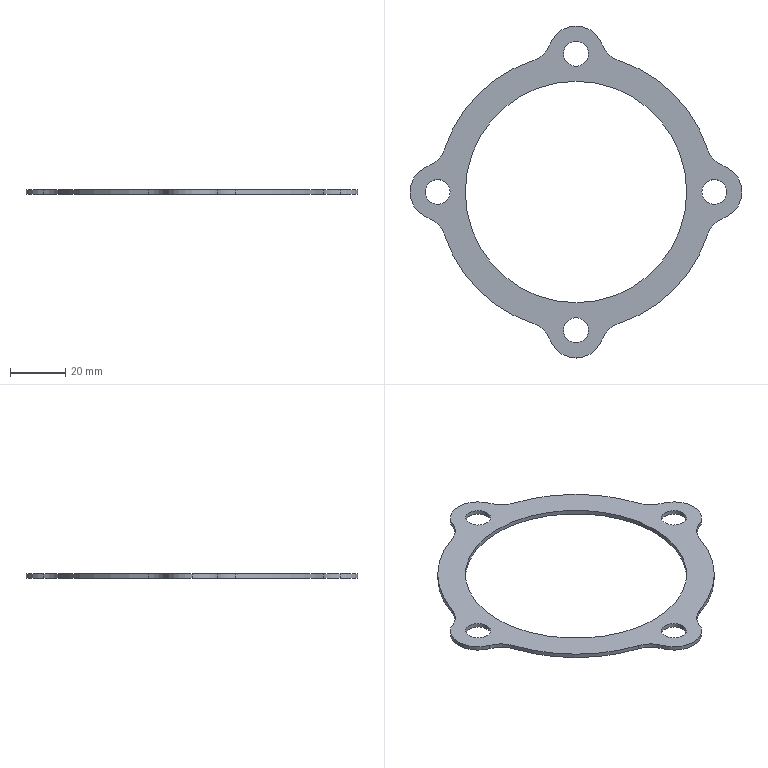Part | SolidWorks | features Extrusion 1 | 1 solid | 29 faces | box 120 x 120 x 1.5 mm | volume 4907 mm3 | cylinder 27 | plane 2 | commonest cylinder face diameters 20 x13 9 x8 100 x4 80 x2
STEP:
#1=CARTESIAN_POINT('',(45.5,0.,1.5));
#2=VERTEX_POINT('',#1);
#3=CARTESIAN_POINT('',(54.5,0.,1.5));
#4=VERTEX_POINT('',#3);
#5=CARTESIAN_POINT('',(50.,0.,1.5));
#6=DIRECTION('',(0.,0.,1.));
#7=DIRECTION('',(1.,0.,0.));
#8=AXIS2_PLACEMENT_3D('',#5,#6,#7);
#9=CIRCLE('',#8,4.5);
#10=EDGE_CURVE('',#2,#4,#9,.T.);
#11=ORIENTED_EDGE('',*,*,#10,.T.);
#12=CARTESIAN_POINT('',(54.5,0.,0.));
#13=VERTEX_POINT('',#12);
#14=CARTESIAN_POINT('',(54.5,0.,1.5));
#15=DIRECTION('',(0.,0.,-1.));
#16=VECTOR('',#15,1000.);
#17=LINE('',#14,#16);
#18=EDGE_CURVE('',#4,#13,#17,.T.);
#19=ORIENTED_EDGE('',*,*,#18,.T.);
#20=CARTESIAN_POINT('',(45.5,0.,0.));
#21=VERTEX_POINT('',#20);
#22=CARTESIAN_POINT('',(50.,0.,0.));
#23=DIRECTION('',(0.,0.,1.));
#24=DIRECTION('',(1.,0.,0.));
#25=AXIS2_PLACEMENT_3D('',#22,#23,#24);
#26=CIRCLE('',#25,4.5);
#27=EDGE_CURVE('',#21,#13,#26,.T.);
#28=ORIENTED_EDGE('',*,*,#27,.F.);
#29=CARTESIAN_POINT('',(45.5,0.,1.5));
#30=DIRECTION('',(0.,0.,-1.));
#31=VECTOR('',#30,1000.);
#32=LINE('',#29,#31);
#33=EDGE_CURVE('',#2,#21,#32,.T.);
#34=ORIENTED_EDGE('',*,*,#33,.F.);
#35=EDGE_LOOP('',(#11,#19,#28,#34));
#36=FACE_OUTER_BOUND('',#35,.T.);
#37=CARTESIAN_POINT('',(50.,0.,1.5));
#38=DIRECTION('',(0.,0.,-1.));
#39=DIRECTION('',(-1.,0.,0.));
#40=AXIS2_PLACEMENT_3D('',#37,#38,#39);
#41=CYLINDRICAL_SURFACE('',#40,4.5);
#42=ADVANCED_FACE('',(#36),#41,.F.);
#43=CARTESIAN_POINT('',(-4.5,-50.,1.5));
#44=VERTEX_POINT('',#43);
#45=CARTESIAN_POINT('',(4.5,-50.,1.5));
#46=VERTEX_POINT('',#45);
#47=CARTESIAN_POINT('',(0.,-50.,1.5));
#48=DIRECTION('',(0.,0.,1.));
#49=DIRECTION('',(1.,0.,0.));
#50=AXIS2_PLACEMENT_3D('',#47,#48,#49);
#51=CIRCLE('',#50,4.5);
#52=EDGE_CURVE('',#44,#46,#51,.T.);
#53=ORIENTED_EDGE('',*,*,#52,.T.);
#54=CARTESIAN_POINT('',(4.5,-50.,0.));
#55=VERTEX_POINT('',#54);
#56=CARTESIAN_POINT('',(4.5,-50.,1.5));
#57=DIRECTION('',(0.,0.,-1.));
#58=VECTOR('',#57,1000.);
#59=LINE('',#56,#58);
#60=EDGE_CURVE('',#46,#55,#59,.T.);
#61=ORIENTED_EDGE('',*,*,#60,.T.);
#62=CARTESIAN_POINT('',(-4.5,-50.,0.));
#63=VERTEX_POINT('',#62);
#64=CARTESIAN_POINT('',(0.,-50.,0.));
#65=DIRECTION('',(0.,0.,1.));
#66=DIRECTION('',(1.,0.,0.));
#67=AXIS2_PLACEMENT_3D('',#64,#65,#66);
#68=CIRCLE('',#67,4.5);
#69=EDGE_CURVE('',#63,#55,#68,.T.);
#70=ORIENTED_EDGE('',*,*,#69,.F.);
#71=CARTESIAN_POINT('',(-4.5,-50.,1.5));
#72=DIRECTION('',(0.,0.,-1.));
#73=VECTOR('',#72,1000.);
#74=LINE('',#71,#73);
#75=EDGE_CURVE('',#44,#63,#74,.T.);
#76=ORIENTED_EDGE('',*,*,#75,.F.);
#77=EDGE_LOOP('',(#53,#61,#70,#76));
#78=FACE_OUTER_BOUND('',#77,.T.);
#79=CARTESIAN_POINT('',(0.,-50.,1.5));
#80=DIRECTION('',(0.,0.,-1.));
#81=DIRECTION('',(-1.,0.,0.));
#82=AXIS2_PLACEMENT_3D('',#79,#80,#81);
#83=CYLINDRICAL_SURFACE('',#82,4.5);
#84=ADVANCED_FACE('',(#78),#83,.F.);
#85=CARTESIAN_POINT('',(-54.5,0.,1.5));
#86=VERTEX_POINT('',#85);
#87=CARTESIAN_POINT('',(-45.5,0.,1.5));
#88=VERTEX_POINT('',#87);
#89=CARTESIAN_POINT('',(-50.,0.,1.5));
#90=DIRECTION('',(0.,0.,1.));
#91=DIRECTION('',(1.,0.,0.));
#92=AXIS2_PLACEMENT_3D('',#89,#90,#91);
#93=CIRCLE('',#92,4.5);
#94=EDGE_CURVE('',#86,#88,#93,.T.);
#95=ORIENTED_EDGE('',*,*,#94,.T.);
#96=CARTESIAN_POINT('',(-45.5,0.,0.));
#97=VERTEX_POINT('',#96);
#98=CARTESIAN_POINT('',(-45.5,0.,1.5));
#99=DIRECTION('',(0.,0.,-1.));
#100=VECTOR('',#99,1000.);
#101=LINE('',#98,#100);
#102=EDGE_CURVE('',#88,#97,#101,.T.);
#103=ORIENTED_EDGE('',*,*,#102,.T.);
#104=CARTESIAN_POINT('',(-54.5,0.,0.));
#105=VERTEX_POINT('',#104);
#106=CARTESIAN_POINT('',(-50.,0.,0.));
#107=DIRECTION('',(0.,0.,1.));
#108=DIRECTION('',(1.,0.,0.));
#109=AXIS2_PLACEMENT_3D('',#106,#107,#108);
#110=CIRCLE('',#109,4.5);
#111=EDGE_CURVE('',#105,#97,#110,.T.);
#112=ORIENTED_EDGE('',*,*,#111,.F.);
#113=CARTESIAN_POINT('',(-54.5,0.,1.5));
#114=DIRECTION('',(0.,0.,-1.));
#115=VECTOR('',#114,1000.);
#116=LINE('',#113,#115);
#117=EDGE_CURVE('',#86,#105,#116,.T.);
#118=ORIENTED_EDGE('',*,*,#117,.F.);
#119=EDGE_LOOP('',(#95,#103,#112,#118));
#120=FACE_OUTER_BOUND('',#119,.T.);
#121=CARTESIAN_POINT('',(-50.,0.,1.5));
#122=DIRECTION('',(0.,0.,-1.));
#123=DIRECTION('',(-1.,0.,0.));
#124=AXIS2_PLACEMENT_3D('',#121,#122,#123);
#125=CYLINDRICAL_SURFACE('',#124,4.5);
#126=ADVANCED_FACE('',(#120),#125,.F.);
#127=CARTESIAN_POINT('',(-4.5,50.,1.5));
#128=VERTEX_POINT('',#127);
#129=CARTESIAN_POINT('',(4.5,50.,1.5));
#130=VERTEX_POINT('',#129);
#131=CARTESIAN_POINT('',(0.,50.,1.5));
#132=DIRECTION('',(0.,0.,1.));
#133=DIRECTION('',(1.,0.,0.));
#134=AXIS2_PLACEMENT_3D('',#131,#132,#133);
#135=CIRCLE('',#134,4.5);
#136=EDGE_CURVE('',#128,#130,#135,.T.);
#137=ORIENTED_EDGE('',*,*,#136,.T.);
#138=CARTESIAN_POINT('',(4.5,50.,0.));
#139=VERTEX_POINT('',#138);
#140=CARTESIAN_POINT('',(4.5,50.,1.5));
#141=DIRECTION('',(0.,0.,-1.));
#142=VECTOR('',#141,1000.);
#143=LINE('',#140,#142);
#144=EDGE_CURVE('',#130,#139,#143,.T.);
#145=ORIENTED_EDGE('',*,*,#144,.T.);
#146=CARTESIAN_POINT('',(-4.5,50.,0.));
#147=VERTEX_POINT('',#146);
#148=CARTESIAN_POINT('',(0.,50.,0.));
#149=DIRECTION('',(0.,0.,1.));
#150=DIRECTION('',(1.,0.,0.));
#151=AXIS2_PLACEMENT_3D('',#148,#149,#150);
#152=CIRCLE('',#151,4.5);
#153=EDGE_CURVE('',#147,#139,#152,.T.);
#154=ORIENTED_EDGE('',*,*,#153,.F.);
#155=CARTESIAN_POINT('',(-4.5,50.,1.5));
#156=DIRECTION('',(0.,0.,-1.));
#157=VECTOR('',#156,1000.);
#158=LINE('',#155,#157);
#159=EDGE_CURVE('',#128,#147,#158,.T.);
#160=ORIENTED_EDGE('',*,*,#159,.F.);
#161=EDGE_LOOP('',(#137,#145,#154,#160));
#162=FACE_OUTER_BOUND('',#161,.T.);
#163=CARTESIAN_POINT('',(0.,50.,1.5));
#164=DIRECTION('',(0.,0.,-1.));
#165=DIRECTION('',(-1.,0.,0.));
#166=AXIS2_PLACEMENT_3D('',#163,#164,#165);
#167=CYLINDRICAL_SURFACE('',#166,4.5);
#168=ADVANCED_FACE('',(#162),#167,.F.);
#169=CARTESIAN_POINT('',(-40.,0.,1.5));
#170=VERTEX_POINT('',#169);
#171=CARTESIAN_POINT('',(40.,0.,1.5));
#172=VERTEX_POINT('',#171);
#173=CARTESIAN_POINT('',(0.,0.,1.5));
#174=DIRECTION('',(0.,0.,1.));
#175=DIRECTION('',(1.,0.,0.));
#176=AXIS2_PLACEMENT_3D('',#173,#174,#175);
#177=CIRCLE('',#176,40.);
#178=EDGE_CURVE('',#170,#172,#177,.T.);
#179=ORIENTED_EDGE('',*,*,#178,.T.);
#180=CARTESIAN_POINT('',(40.,0.,0.));
#181=VERTEX_POINT('',#180);
#182=CARTESIAN_POINT('',(40.,0.,1.5));
#183=DIRECTION('',(0.,0.,-1.));
#184=VECTOR('',#183,1000.);
#185=LINE('',#182,#184);
#186=EDGE_CURVE('',#172,#181,#185,.T.);
#187=ORIENTED_EDGE('',*,*,#186,.T.);
#188=CARTESIAN_POINT('',(-40.,0.,0.));
#189=VERTEX_POINT('',#188);
#190=CARTESIAN_POINT('',(0.,0.,0.));
#191=DIRECTION('',(0.,0.,1.));
#192=DIRECTION('',(1.,0.,0.));
#193=AXIS2_PLACEMENT_3D('',#190,#191,#192);
#194=CIRCLE('',#193,40.);
#195=EDGE_CURVE('',#189,#181,#194,.T.);
#196=ORIENTED_EDGE('',*,*,#195,.F.);
#197=CARTESIAN_POINT('',(-40.,0.,1.5));
#198=DIRECTION('',(0.,0.,-1.));
#199=VECTOR('',#198,1000.);
#200=LINE('',#197,#199);
#201=EDGE_CURVE('',#170,#189,#200,.T.);
#202=ORIENTED_EDGE('',*,*,#201,.F.);
#203=EDGE_LOOP('',(#179,#187,#196,#202));
#204=FACE_OUTER_BOUND('',#203,.T.);
#205=CARTESIAN_POINT('',(0.,0.,1.5));
#206=DIRECTION('',(0.,0.,-1.));
#207=DIRECTION('',(-1.,0.,0.));
#208=AXIS2_PLACEMENT_3D('',#205,#206,#207);
#209=CYLINDRICAL_SURFACE('',#208,40.);
#210=ADVANCED_FACE('',(#204),#209,.F.);
#211=CARTESIAN_POINT('',(-60.,0.,1.5));
#212=VERTEX_POINT('',#211);
#213=CARTESIAN_POINT('',(-53.5,-9.367,1.5));
#214=VERTEX_POINT('',#213);
#215=CARTESIAN_POINT('',(-50.,0.,1.5));
#216=DIRECTION('',(0.,0.,1.));
#217=DIRECTION('',(1.,0.,0.));
#218=AXIS2_PLACEMENT_3D('',#215,#216,#217);
#219=CIRCLE('',#218,10.);
#220=EDGE_CURVE('',#212,#214,#219,.T.);
#221=ORIENTED_EDGE('',*,*,#220,.F.);
#222=CARTESIAN_POINT('',(-60.,0.,0.));
#223=VERTEX_POINT('',#222);
#224=CARTESIAN_POINT('',(-60.,0.,1.5));
#225=DIRECTION('',(0.,0.,-1.));
#226=VECTOR('',#225,1000.);
#227=LINE('',#224,#226);
#228=EDGE_CURVE('',#212,#223,#227,.T.);
#229=ORIENTED_EDGE('',*,*,#228,.T.);
#230=CARTESIAN_POINT('',(-53.5,-9.367,0.));
#231=VERTEX_POINT('',#230);
#232=CARTESIAN_POINT('',(-50.,0.,0.));
#233=DIRECTION('',(0.,0.,1.));
#234=DIRECTION('',(1.,0.,0.));
#235=AXIS2_PLACEMENT_3D('',#232,#233,#234);
#236=CIRCLE('',#235,10.);
#237=EDGE_CURVE('',#223,#231,#236,.T.);
#238=ORIENTED_EDGE('',*,*,#237,.T.);
#239=CARTESIAN_POINT('',(-53.5,-9.367,1.5));
#240=DIRECTION('',(0.,0.,-1.));
#241=VECTOR('',#240,1000.);
#242=LINE('',#239,#241);
#243=EDGE_CURVE('',#214,#231,#242,.T.);
#244=ORIENTED_EDGE('',*,*,#243,.F.);
#245=EDGE_LOOP('',(#221,#229,#238,#244));
#246=FACE_OUTER_BOUND('',#245,.T.);
#247=CARTESIAN_POINT('',(-50.,0.,1.5));
#248=DIRECTION('',(0.,0.,-1.));
#249=DIRECTION('',(-1.,0.,0.));
#250=AXIS2_PLACEMENT_3D('',#247,#248,#249);
#251=CYLINDRICAL_SURFACE('',#250,10.);
#252=ADVANCED_FACE('',(#246),#251,.T.);
#253=ORIENTED_EDGE('',*,*,#52,.F.);
#254=CARTESIAN_POINT('',(0.,-50.,1.5));
#255=DIRECTION('',(0.,0.,1.));
#256=DIRECTION('',(1.,0.,0.));
#257=AXIS2_PLACEMENT_3D('',#254,#255,#256);
#258=CIRCLE('',#257,4.5);
#259=EDGE_CURVE('',#46,#44,#258,.T.);
#260=ORIENTED_EDGE('',*,*,#259,.F.);
#261=EDGE_LOOP('',(#253,#260));
#262=FACE_BOUND('',#261,.T.);
#263=ORIENTED_EDGE('',*,*,#136,.F.);
#264=CARTESIAN_POINT('',(0.,50.,1.5));
#265=DIRECTION('',(0.,0.,1.));
#266=DIRECTION('',(1.,0.,0.));
#267=AXIS2_PLACEMENT_3D('',#264,#265,#266);
#268=CIRCLE('',#267,4.5);
#269=EDGE_CURVE('',#130,#128,#268,.T.);
#270=ORIENTED_EDGE('',*,*,#269,.F.);
#271=EDGE_LOOP('',(#263,#270));
#272=FACE_BOUND('',#271,.T.);
#273=CARTESIAN_POINT('',(-9.367,53.5,1.5));
#274=VERTEX_POINT('',#273);
#275=CARTESIAN_POINT('',(-15.612,47.5,1.5));
#276=VERTEX_POINT('',#275);
#277=CARTESIAN_POINT('',(-18.735,57.,1.5));
#278=DIRECTION('',(0.,0.,-1.));
#279=DIRECTION('',(1.,0.,0.));
#280=AXIS2_PLACEMENT_3D('',#277,#278,#279);
#281=CIRCLE('',#280,10.);
#282=EDGE_CURVE('',#274,#276,#281,.T.);
#283=ORIENTED_EDGE('',*,*,#282,.T.);
#284=CARTESIAN_POINT('',(-47.5,15.612,1.5));
#285=VERTEX_POINT('',#284);
#286=CARTESIAN_POINT('',(0.,0.,1.5));
#287=DIRECTION('',(0.,0.,1.));
#288=DIRECTION('',(1.,0.,0.));
#289=AXIS2_PLACEMENT_3D('',#286,#287,#288);
#290=CIRCLE('',#289,50.);
#291=EDGE_CURVE('',#276,#285,#290,.T.);
#292=ORIENTED_EDGE('',*,*,#291,.T.);
#293=CARTESIAN_POINT('',(-53.5,9.367,1.5));
#294=VERTEX_POINT('',#293);
#295=CARTESIAN_POINT('',(-57.,18.735,1.5));
#296=DIRECTION('',(0.,0.,-1.));
#297=DIRECTION('',(-1.,0.,0.));
#298=AXIS2_PLACEMENT_3D('',#295,#296,#297);
#299=CIRCLE('',#298,10.);
#300=EDGE_CURVE('',#285,#294,#299,.T.);
#301=ORIENTED_EDGE('',*,*,#300,.T.);
#302=CARTESIAN_POINT('',(-50.,0.,1.5));
#303=DIRECTION('',(0.,0.,1.));
#304=DIRECTION('',(1.,0.,0.));
#305=AXIS2_PLACEMENT_3D('',#302,#303,#304);
#306=CIRCLE('',#305,10.);
#307=EDGE_CURVE('',#294,#212,#306,.T.);
#308=ORIENTED_EDGE('',*,*,#307,.T.);
#309=ORIENTED_EDGE('',*,*,#220,.T.);
#310=CARTESIAN_POINT('',(-47.5,-15.612,1.5));
#311=VERTEX_POINT('',#310);
#312=CARTESIAN_POINT('',(-57.,-18.735,1.5));
#313=DIRECTION('',(0.,0.,-1.));
#314=DIRECTION('',(-1.,0.,0.));
#315=AXIS2_PLACEMENT_3D('',#312,#313,#314);
#316=CIRCLE('',#315,10.);
#317=EDGE_CURVE('',#214,#311,#316,.T.);
#318=ORIENTED_EDGE('',*,*,#317,.T.);
#319=CARTESIAN_POINT('',(-15.612,-47.5,1.5));
#320=VERTEX_POINT('',#319);
#321=CARTESIAN_POINT('',(0.,0.,1.5));
#322=DIRECTION('',(0.,0.,1.));
#323=DIRECTION('',(1.,0.,0.));
#324=AXIS2_PLACEMENT_3D('',#321,#322,#323);
#325=CIRCLE('',#324,50.);
#326=EDGE_CURVE('',#311,#320,#325,.T.);
#327=ORIENTED_EDGE('',*,*,#326,.T.);
#328=CARTESIAN_POINT('',(-9.367,-53.5,1.5));
#329=VERTEX_POINT('',#328);
#330=CARTESIAN_POINT('',(-18.735,-57.,1.5));
#331=DIRECTION('',(0.,0.,-1.));
#332=DIRECTION('',(-1.,0.,0.));
#333=AXIS2_PLACEMENT_3D('',#330,#331,#332);
#334=CIRCLE('',#333,10.);
#335=EDGE_CURVE('',#320,#329,#334,.T.);
#336=ORIENTED_EDGE('',*,*,#335,.T.);
#337=CARTESIAN_POINT('',(9.367,-53.5,1.5));
#338=VERTEX_POINT('',#337);
#339=CARTESIAN_POINT('',(0.,-50.,1.5));
#340=DIRECTION('',(0.,0.,1.));
#341=DIRECTION('',(1.,0.,0.));
#342=AXIS2_PLACEMENT_3D('',#339,#340,#341);
#343=CIRCLE('',#342,10.);
#344=EDGE_CURVE('',#329,#338,#343,.T.);
#345=ORIENTED_EDGE('',*,*,#344,.T.);
#346=CARTESIAN_POINT('',(15.612,-47.5,1.5));
#347=VERTEX_POINT('',#346);
#348=CARTESIAN_POINT('',(18.735,-57.,1.5));
#349=DIRECTION('',(0.,0.,-1.));
#350=DIRECTION('',(-1.,0.,0.));
#351=AXIS2_PLACEMENT_3D('',#348,#349,#350);
#352=CIRCLE('',#351,10.);
#353=EDGE_CURVE('',#338,#347,#352,.T.);
#354=ORIENTED_EDGE('',*,*,#353,.T.);
#355=CARTESIAN_POINT('',(47.5,-15.612,1.5));
#356=VERTEX_POINT('',#355);
#357=CARTESIAN_POINT('',(0.,0.,1.5));
#358=DIRECTION('',(0.,0.,1.));
#359=DIRECTION('',(1.,0.,0.));
#360=AXIS2_PLACEMENT_3D('',#357,#358,#359);
#361=CIRCLE('',#360,50.);
#362=EDGE_CURVE('',#347,#356,#361,.T.);
#363=ORIENTED_EDGE('',*,*,#362,.T.);
#364=CARTESIAN_POINT('',(53.5,-9.367,1.5));
#365=VERTEX_POINT('',#364);
#366=CARTESIAN_POINT('',(57.,-18.735,1.5));
#367=DIRECTION('',(0.,0.,-1.));
#368=DIRECTION('',(-1.,0.,0.));
#369=AXIS2_PLACEMENT_3D('',#366,#367,#368);
#370=CIRCLE('',#369,10.);
#371=EDGE_CURVE('',#356,#365,#370,.T.);
#372=ORIENTED_EDGE('',*,*,#371,.T.);
#373=CARTESIAN_POINT('',(53.5,9.367,1.5));
#374=VERTEX_POINT('',#373);
#375=CARTESIAN_POINT('',(50.,0.,1.5));
#376=DIRECTION('',(0.,0.,1.));
#377=DIRECTION('',(1.,0.,0.));
#378=AXIS2_PLACEMENT_3D('',#375,#376,#377);
#379=CIRCLE('',#378,10.);
#380=EDGE_CURVE('',#365,#374,#379,.T.);
#381=ORIENTED_EDGE('',*,*,#380,.T.);
#382=CARTESIAN_POINT('',(47.5,15.612,1.5));
#383=VERTEX_POINT('',#382);
#384=CARTESIAN_POINT('',(57.,18.735,1.5));
#385=DIRECTION('',(0.,0.,-1.));
#386=DIRECTION('',(-1.,0.,0.));
#387=AXIS2_PLACEMENT_3D('',#384,#385,#386);
#388=CIRCLE('',#387,10.);
#389=EDGE_CURVE('',#374,#383,#388,.T.);
#390=ORIENTED_EDGE('',*,*,#389,.T.);
#391=CARTESIAN_POINT('',(15.612,47.5,1.5));
#392=VERTEX_POINT('',#391);
#393=CARTESIAN_POINT('',(0.,0.,1.5));
#394=DIRECTION('',(0.,0.,1.));
#395=DIRECTION('',(1.,0.,0.));
#396=AXIS2_PLACEMENT_3D('',#393,#394,#395);
#397=CIRCLE('',#396,50.);
#398=EDGE_CURVE('',#383,#392,#397,.T.);
#399=ORIENTED_EDGE('',*,*,#398,.T.);
#400=CARTESIAN_POINT('',(9.367,53.5,1.5));
#401=VERTEX_POINT('',#400);
#402=CARTESIAN_POINT('',(18.735,57.,1.5));
#403=DIRECTION('',(0.,0.,-1.));
#404=DIRECTION('',(-1.,0.,0.));
#405=AXIS2_PLACEMENT_3D('',#402,#403,#404);
#406=CIRCLE('',#405,10.);
#407=EDGE_CURVE('',#392,#401,#406,.T.);
#408=ORIENTED_EDGE('',*,*,#407,.T.);
#409=CARTESIAN_POINT('',(0.,50.,1.5));
#410=DIRECTION('',(0.,0.,1.));
#411=DIRECTION('',(1.,0.,0.));
#412=AXIS2_PLACEMENT_3D('',#409,#410,#411);
#413=CIRCLE('',#412,10.);
#414=EDGE_CURVE('',#401,#274,#413,.T.);
#415=ORIENTED_EDGE('',*,*,#414,.T.);
#416=EDGE_LOOP('',(#283,#292,#301,#308,#309,#318,#327,#336,#345,#354,#363,#372,#381,#390,#399,#408,#415));
#417=FACE_OUTER_BOUND('',#416,.T.);
#418=ORIENTED_EDGE('',*,*,#178,.F.);
#419=CARTESIAN_POINT('',(0.,0.,1.5));
#420=DIRECTION('',(0.,0.,1.));
#421=DIRECTION('',(1.,0.,0.));
#422=AXIS2_PLACEMENT_3D('',#419,#420,#421);
#423=CIRCLE('',#422,40.);
#424=EDGE_CURVE('',#172,#170,#423,.T.);
#425=ORIENTED_EDGE('',*,*,#424,.F.);
#426=EDGE_LOOP('',(#418,#425));
#427=FACE_BOUND('',#426,.T.);
#428=ORIENTED_EDGE('',*,*,#94,.F.);
#429=CARTESIAN_POINT('',(-50.,0.,1.5));
#430=DIRECTION('',(0.,0.,1.));
#431=DIRECTION('',(1.,0.,0.));
#432=AXIS2_PLACEMENT_3D('',#429,#430,#431);
#433=CIRCLE('',#432,4.5);
#434=EDGE_CURVE('',#88,#86,#433,.T.);
#435=ORIENTED_EDGE('',*,*,#434,.F.);
#436=EDGE_LOOP('',(#428,#435));
#437=FACE_BOUND('',#436,.T.);
#438=ORIENTED_EDGE('',*,*,#10,.F.);
#439=CARTESIAN_POINT('',(50.,0.,1.5));
#440=DIRECTION('',(0.,0.,1.));
#441=DIRECTION('',(1.,0.,0.));
#442=AXIS2_PLACEMENT_3D('',#439,#440,#441);
#443=CIRCLE('',#442,4.5);
#444=EDGE_CURVE('',#4,#2,#443,.T.);
#445=ORIENTED_EDGE('',*,*,#444,.F.);
#446=EDGE_LOOP('',(#438,#445));
#447=FACE_BOUND('',#446,.T.);
#448=CARTESIAN_POINT('',(-9.367,53.5,1.5));
#449=DIRECTION('',(0.,0.,1.));
#450=DIRECTION('',(1.,0.,0.));
#451=AXIS2_PLACEMENT_3D('',#448,#449,#450);
#452=PLANE('',#451);
#453=ADVANCED_FACE('',(#262,#272,#417,#427,#437,#447),#452,.T.);
#454=CARTESIAN_POINT('',(-9.367,53.5,0.));
#455=VERTEX_POINT('',#454);
#456=CARTESIAN_POINT('',(-15.612,47.5,0.));
#457=VERTEX_POINT('',#456);
#458=CARTESIAN_POINT('',(-18.735,57.,0.));
#459=DIRECTION('',(0.,0.,-1.));
#460=DIRECTION('',(1.,0.,0.));
#461=AXIS2_PLACEMENT_3D('',#458,#459,#460);
#462=CIRCLE('',#461,10.);
#463=EDGE_CURVE('',#455,#457,#462,.T.);
#464=ORIENTED_EDGE('',*,*,#463,.F.);
#465=CARTESIAN_POINT('',(9.367,53.5,0.));
#466=VERTEX_POINT('',#465);
#467=CARTESIAN_POINT('',(0.,50.,0.));
#468=DIRECTION('',(0.,0.,1.));
#469=DIRECTION('',(1.,0.,0.));
#470=AXIS2_PLACEMENT_3D('',#467,#468,#469);
#471=CIRCLE('',#470,10.);
#472=EDGE_CURVE('',#466,#455,#471,.T.);
#473=ORIENTED_EDGE('',*,*,#472,.F.);
#474=CARTESIAN_POINT('',(15.612,47.5,0.));
#475=VERTEX_POINT('',#474);
#476=CARTESIAN_POINT('',(18.735,57.,0.));
#477=DIRECTION('',(0.,0.,-1.));
#478=DIRECTION('',(-1.,0.,0.));
#479=AXIS2_PLACEMENT_3D('',#476,#477,#478);
#480=CIRCLE('',#479,10.);
#481=EDGE_CURVE('',#475,#466,#480,.T.);
#482=ORIENTED_EDGE('',*,*,#481,.F.);
#483=CARTESIAN_POINT('',(47.5,15.612,0.));
#484=VERTEX_POINT('',#483);
#485=CARTESIAN_POINT('',(0.,0.,0.));
#486=DIRECTION('',(0.,0.,1.));
#487=DIRECTION('',(1.,0.,0.));
#488=AXIS2_PLACEMENT_3D('',#485,#486,#487);
#489=CIRCLE('',#488,50.);
#490=EDGE_CURVE('',#484,#475,#489,.T.);
#491=ORIENTED_EDGE('',*,*,#490,.F.);
#492=CARTESIAN_POINT('',(53.5,9.367,0.));
#493=VERTEX_POINT('',#492);
#494=CARTESIAN_POINT('',(57.,18.735,0.));
#495=DIRECTION('',(0.,0.,-1.));
#496=DIRECTION('',(-1.,0.,0.));
#497=AXIS2_PLACEMENT_3D('',#494,#495,#496);
#498=CIRCLE('',#497,10.);
#499=EDGE_CURVE('',#493,#484,#498,.T.);
#500=ORIENTED_EDGE('',*,*,#499,.F.);
#501=CARTESIAN_POINT('',(53.5,-9.367,0.));
#502=VERTEX_POINT('',#501);
#503=CARTESIAN_POINT('',(50.,0.,0.));
#504=DIRECTION('',(0.,0.,1.));
#505=DIRECTION('',(1.,0.,0.));
#506=AXIS2_PLACEMENT_3D('',#503,#504,#505);
#507=CIRCLE('',#506,10.);
#508=EDGE_CURVE('',#502,#493,#507,.T.);
#509=ORIENTED_EDGE('',*,*,#508,.F.);
#510=CARTESIAN_POINT('',(47.5,-15.612,0.));
#511=VERTEX_POINT('',#510);
#512=CARTESIAN_POINT('',(57.,-18.735,0.));
#513=DIRECTION('',(0.,0.,-1.));
#514=DIRECTION('',(-1.,0.,0.));
#515=AXIS2_PLACEMENT_3D('',#512,#513,#514);
#516=CIRCLE('',#515,10.);
#517=EDGE_CURVE('',#511,#502,#516,.T.);
#518=ORIENTED_EDGE('',*,*,#517,.F.);
#519=CARTESIAN_POINT('',(15.612,-47.5,0.));
#520=VERTEX_POINT('',#519);
#521=CARTESIAN_POINT('',(0.,0.,0.));
#522=DIRECTION('',(0.,0.,1.));
#523=DIRECTION('',(1.,0.,0.));
#524=AXIS2_PLACEMENT_3D('',#521,#522,#523);
#525=CIRCLE('',#524,50.);
#526=EDGE_CURVE('',#520,#511,#525,.T.);
#527=ORIENTED_EDGE('',*,*,#526,.F.);
#528=CARTESIAN_POINT('',(9.367,-53.5,0.));
#529=VERTEX_POINT('',#528);
#530=CARTESIAN_POINT('',(18.735,-57.,0.));
#531=DIRECTION('',(0.,0.,-1.));
#532=DIRECTION('',(-1.,0.,0.));
#533=AXIS2_PLACEMENT_3D('',#530,#531,#532);
#534=CIRCLE('',#533,10.);
#535=EDGE_CURVE('',#529,#520,#534,.T.);
#536=ORIENTED_EDGE('',*,*,#535,.F.);
#537=CARTESIAN_POINT('',(-9.367,-53.5,0.));
#538=VERTEX_POINT('',#537);
#539=CARTESIAN_POINT('',(0.,-50.,0.));
#540=DIRECTION('',(0.,0.,1.));
#541=DIRECTION('',(1.,0.,0.));
#542=AXIS2_PLACEMENT_3D('',#539,#540,#541);
#543=CIRCLE('',#542,10.);
#544=EDGE_CURVE('',#538,#529,#543,.T.);
#545=ORIENTED_EDGE('',*,*,#544,.F.);
#546=CARTESIAN_POINT('',(-15.612,-47.5,0.));
#547=VERTEX_POINT('',#546);
#548=CARTESIAN_POINT('',(-18.735,-57.,0.));
#549=DIRECTION('',(0.,0.,-1.));
#550=DIRECTION('',(-1.,0.,0.));
#551=AXIS2_PLACEMENT_3D('',#548,#549,#550);
#552=CIRCLE('',#551,10.);
#553=EDGE_CURVE('',#547,#538,#552,.T.);
#554=ORIENTED_EDGE('',*,*,#553,.F.);
#555=CARTESIAN_POINT('',(-47.5,-15.612,0.));
#556=VERTEX_POINT('',#555);
#557=CARTESIAN_POINT('',(0.,0.,0.));
#558=DIRECTION('',(0.,0.,1.));
#559=DIRECTION('',(1.,0.,0.));
#560=AXIS2_PLACEMENT_3D('',#557,#558,#559);
#561=CIRCLE('',#560,50.);
#562=EDGE_CURVE('',#556,#547,#561,.T.);
#563=ORIENTED_EDGE('',*,*,#562,.F.);
#564=CARTESIAN_POINT('',(-57.,-18.735,0.));
#565=DIRECTION('',(0.,0.,-1.));
#566=DIRECTION('',(-1.,0.,0.));
#567=AXIS2_PLACEMENT_3D('',#564,#565,#566);
#568=CIRCLE('',#567,10.);
#569=EDGE_CURVE('',#231,#556,#568,.T.);
#570=ORIENTED_EDGE('',*,*,#569,.F.);
#571=ORIENTED_EDGE('',*,*,#237,.F.);
#572=CARTESIAN_POINT('',(-53.5,9.367,0.));
#573=VERTEX_POINT('',#572);
#574=CARTESIAN_POINT('',(-50.,0.,0.));
#575=DIRECTION('',(0.,0.,1.));
#576=DIRECTION('',(1.,0.,0.));
#577=AXIS2_PLACEMENT_3D('',#574,#575,#576);
#578=CIRCLE('',#577,10.);
#579=EDGE_CURVE('',#573,#223,#578,.T.);
#580=ORIENTED_EDGE('',*,*,#579,.F.);
#581=CARTESIAN_POINT('',(-47.5,15.612,0.));
#582=VERTEX_POINT('',#581);
#583=CARTESIAN_POINT('',(-57.,18.735,0.));
#584=DIRECTION('',(0.,0.,-1.));
#585=DIRECTION('',(-1.,0.,0.));
#586=AXIS2_PLACEMENT_3D('',#583,#584,#585);
#587=CIRCLE('',#586,10.);
#588=EDGE_CURVE('',#582,#573,#587,.T.);
#589=ORIENTED_EDGE('',*,*,#588,.F.);
#590=CARTESIAN_POINT('',(0.,0.,0.));
#591=DIRECTION('',(0.,0.,1.));
#592=DIRECTION('',(1.,0.,0.));
#593=AXIS2_PLACEMENT_3D('',#590,#591,#592);
#594=CIRCLE('',#593,50.);
#595=EDGE_CURVE('',#457,#582,#594,.T.);
#596=ORIENTED_EDGE('',*,*,#595,.F.);
#597=EDGE_LOOP('',(#464,#473,#482,#491,#500,#509,#518,#527,#536,#545,#554,#563,#570,#571,#580,#589,#596));
#598=FACE_OUTER_BOUND('',#597,.T.);
#599=ORIENTED_EDGE('',*,*,#195,.T.);
#600=CARTESIAN_POINT('',(0.,0.,0.));
#601=DIRECTION('',(0.,0.,1.));
#602=DIRECTION('',(1.,0.,0.));
#603=AXIS2_PLACEMENT_3D('',#600,#601,#602);
#604=CIRCLE('',#603,40.);
#605=EDGE_CURVE('',#181,#189,#604,.T.);
#606=ORIENTED_EDGE('',*,*,#605,.T.);
#607=EDGE_LOOP('',(#599,#606));
#608=FACE_BOUND('',#607,.T.);
#609=ORIENTED_EDGE('',*,*,#153,.T.);
#610=CARTESIAN_POINT('',(0.,50.,0.));
#611=DIRECTION('',(0.,0.,1.));
#612=DIRECTION('',(1.,0.,0.));
#613=AXIS2_PLACEMENT_3D('',#610,#611,#612);
#614=CIRCLE('',#613,4.5);
#615=EDGE_CURVE('',#139,#147,#614,.T.);
#616=ORIENTED_EDGE('',*,*,#615,.T.);
#617=EDGE_LOOP('',(#609,#616));
#618=FACE_BOUND('',#617,.T.);
#619=ORIENTED_EDGE('',*,*,#111,.T.);
#620=CARTESIAN_POINT('',(-50.,0.,0.));
#621=DIRECTION('',(0.,0.,1.));
#622=DIRECTION('',(1.,0.,0.));
#623=AXIS2_PLACEMENT_3D('',#620,#621,#622);
#624=CIRCLE('',#623,4.5);
#625=EDGE_CURVE('',#97,#105,#624,.T.);
#626=ORIENTED_EDGE('',*,*,#625,.T.);
#627=EDGE_LOOP('',(#619,#626));
#628=FACE_BOUND('',#627,.T.);
#629=ORIENTED_EDGE('',*,*,#69,.T.);
#630=CARTESIAN_POINT('',(0.,-50.,0.));
#631=DIRECTION('',(0.,0.,1.));
#632=DIRECTION('',(1.,0.,0.));
#633=AXIS2_PLACEMENT_3D('',#630,#631,#632);
#634=CIRCLE('',#633,4.5);
#635=EDGE_CURVE('',#55,#63,#634,.T.);
#636=ORIENTED_EDGE('',*,*,#635,.T.);
#637=EDGE_LOOP('',(#629,#636));
#638=FACE_BOUND('',#637,.T.);
#639=ORIENTED_EDGE('',*,*,#27,.T.);
#640=CARTESIAN_POINT('',(50.,0.,0.));
#641=DIRECTION('',(0.,0.,1.));
#642=DIRECTION('',(1.,0.,0.));
#643=AXIS2_PLACEMENT_3D('',#640,#641,#642);
#644=CIRCLE('',#643,4.5);
#645=EDGE_CURVE('',#13,#21,#644,.T.);
#646=ORIENTED_EDGE('',*,*,#645,.T.);
#647=EDGE_LOOP('',(#639,#646));
#648=FACE_BOUND('',#647,.T.);
#649=CARTESIAN_POINT('',(-9.367,53.5,0.));
#650=DIRECTION('',(0.,0.,1.));
#651=DIRECTION('',(1.,0.,0.));
#652=AXIS2_PLACEMENT_3D('',#649,#650,#651);
#653=PLANE('',#652);
#654=ADVANCED_FACE('',(#598,#608,#618,#628,#638,#648),#653,.F.);
#655=ORIENTED_EDGE('',*,*,#463,.T.);
#656=CARTESIAN_POINT('',(-15.612,47.5,1.5));
#657=DIRECTION('',(0.,0.,-1.));
#658=VECTOR('',#657,1000.);
#659=LINE('',#656,#658);
#660=EDGE_CURVE('',#276,#457,#659,.T.);
#661=ORIENTED_EDGE('',*,*,#660,.F.);
#662=ORIENTED_EDGE('',*,*,#282,.F.);
#663=CARTESIAN_POINT('',(-9.367,53.5,1.5));
#664=DIRECTION('',(0.,0.,-1.));
#665=VECTOR('',#664,1000.);
#666=LINE('',#663,#665);
#667=EDGE_CURVE('',#274,#455,#666,.T.);
#668=ORIENTED_EDGE('',*,*,#667,.T.);
#669=EDGE_LOOP('',(#655,#661,#662,#668));
#670=FACE_OUTER_BOUND('',#669,.T.);
#671=CARTESIAN_POINT('',(-18.735,57.,1.5));
#672=DIRECTION('',(0.,0.,-1.));
#673=DIRECTION('',(-1.,0.,0.));
#674=AXIS2_PLACEMENT_3D('',#671,#672,#673);
#675=CYLINDRICAL_SURFACE('',#674,10.);
#676=ADVANCED_FACE('',(#670),#675,.F.);
#677=ORIENTED_EDGE('',*,*,#595,.T.);
#678=CARTESIAN_POINT('',(-47.5,15.612,1.5));
#679=DIRECTION('',(0.,0.,-1.));
#680=VECTOR('',#679,1000.);
#681=LINE('',#678,#680);
#682=EDGE_CURVE('',#285,#582,#681,.T.);
#683=ORIENTED_EDGE('',*,*,#682,.F.);
#684=ORIENTED_EDGE('',*,*,#291,.F.);
#685=ORIENTED_EDGE('',*,*,#660,.T.);
#686=EDGE_LOOP('',(#677,#683,#684,#685));
#687=FACE_OUTER_BOUND('',#686,.T.);
#688=CARTESIAN_POINT('',(0.,0.,1.5));
#689=DIRECTION('',(0.,0.,-1.));
#690=DIRECTION('',(-1.,0.,0.));
#691=AXIS2_PLACEMENT_3D('',#688,#689,#690);
#692=CYLINDRICAL_SURFACE('',#691,50.);
#693=ADVANCED_FACE('',(#687),#692,.T.);
#694=ORIENTED_EDGE('',*,*,#588,.T.);
#695=CARTESIAN_POINT('',(-53.5,9.367,1.5));
#696=DIRECTION('',(0.,0.,-1.));
#697=VECTOR('',#696,1000.);
#698=LINE('',#695,#697);
#699=EDGE_CURVE('',#294,#573,#698,.T.);
#700=ORIENTED_EDGE('',*,*,#699,.F.);
#701=ORIENTED_EDGE('',*,*,#300,.F.);
#702=ORIENTED_EDGE('',*,*,#682,.T.);
#703=EDGE_LOOP('',(#694,#700,#701,#702));
#704=FACE_OUTER_BOUND('',#703,.T.);
#705=CARTESIAN_POINT('',(-57.,18.735,1.5));
#706=DIRECTION('',(0.,0.,-1.));
#707=DIRECTION('',(-1.,0.,0.));
#708=AXIS2_PLACEMENT_3D('',#705,#706,#707);
#709=CYLINDRICAL_SURFACE('',#708,10.);
#710=ADVANCED_FACE('',(#704),#709,.F.);
#711=ORIENTED_EDGE('',*,*,#228,.F.);
#712=ORIENTED_EDGE('',*,*,#307,.F.);
#713=ORIENTED_EDGE('',*,*,#699,.T.);
#714=ORIENTED_EDGE('',*,*,#579,.T.);
#715=EDGE_LOOP('',(#711,#712,#713,#714));
#716=FACE_OUTER_BOUND('',#715,.T.);
#717=CARTESIAN_POINT('',(-50.,0.,1.5));
#718=DIRECTION('',(0.,0.,-1.));
#719=DIRECTION('',(-1.,0.,0.));
#720=AXIS2_PLACEMENT_3D('',#717,#718,#719);
#721=CYLINDRICAL_SURFACE('',#720,10.);
#722=ADVANCED_FACE('',(#716),#721,.T.);
#723=ORIENTED_EDGE('',*,*,#569,.T.);
#724=CARTESIAN_POINT('',(-47.5,-15.612,1.5));
#725=DIRECTION('',(0.,0.,-1.));
#726=VECTOR('',#725,1000.);
#727=LINE('',#724,#726);
#728=EDGE_CURVE('',#311,#556,#727,.T.);
#729=ORIENTED_EDGE('',*,*,#728,.F.);
#730=ORIENTED_EDGE('',*,*,#317,.F.);
#731=ORIENTED_EDGE('',*,*,#243,.T.);
#732=EDGE_LOOP('',(#723,#729,#730,#731));
#733=FACE_OUTER_BOUND('',#732,.T.);
#734=CARTESIAN_POINT('',(-57.,-18.735,1.5));
#735=DIRECTION('',(0.,0.,-1.));
#736=DIRECTION('',(-1.,0.,0.));
#737=AXIS2_PLACEMENT_3D('',#734,#735,#736);
#738=CYLINDRICAL_SURFACE('',#737,10.);
#739=ADVANCED_FACE('',(#733),#738,.F.);
#740=ORIENTED_EDGE('',*,*,#562,.T.);
#741=CARTESIAN_POINT('',(-15.612,-47.5,1.5));
#742=DIRECTION('',(0.,0.,-1.));
#743=VECTOR('',#742,1000.);
#744=LINE('',#741,#743);
#745=EDGE_CURVE('',#320,#547,#744,.T.);
#746=ORIENTED_EDGE('',*,*,#745,.F.);
#747=ORIENTED_EDGE('',*,*,#326,.F.);
#748=ORIENTED_EDGE('',*,*,#728,.T.);
#749=EDGE_LOOP('',(#740,#746,#747,#748));
#750=FACE_OUTER_BOUND('',#749,.T.);
#751=CARTESIAN_POINT('',(0.,0.,1.5));
#752=DIRECTION('',(0.,0.,-1.));
#753=DIRECTION('',(-1.,0.,0.));
#754=AXIS2_PLACEMENT_3D('',#751,#752,#753);
#755=CYLINDRICAL_SURFACE('',#754,50.);
#756=ADVANCED_FACE('',(#750),#755,.T.);
#757=ORIENTED_EDGE('',*,*,#553,.T.);
#758=CARTESIAN_POINT('',(-9.367,-53.5,1.5));
#759=DIRECTION('',(0.,0.,-1.));
#760=VECTOR('',#759,1000.);
#761=LINE('',#758,#760);
#762=EDGE_CURVE('',#329,#538,#761,.T.);
#763=ORIENTED_EDGE('',*,*,#762,.F.);
#764=ORIENTED_EDGE('',*,*,#335,.F.);
#765=ORIENTED_EDGE('',*,*,#745,.T.);
#766=EDGE_LOOP('',(#757,#763,#764,#765));
#767=FACE_OUTER_BOUND('',#766,.T.);
#768=CARTESIAN_POINT('',(-18.735,-57.,1.5));
#769=DIRECTION('',(0.,0.,-1.));
#770=DIRECTION('',(-1.,0.,0.));
#771=AXIS2_PLACEMENT_3D('',#768,#769,#770);
#772=CYLINDRICAL_SURFACE('',#771,10.);
#773=ADVANCED_FACE('',(#767),#772,.F.);
#774=ORIENTED_EDGE('',*,*,#544,.T.);
#775=CARTESIAN_POINT('',(9.367,-53.5,1.5));
#776=DIRECTION('',(0.,0.,-1.));
#777=VECTOR('',#776,1000.);
#778=LINE('',#775,#777);
#779=EDGE_CURVE('',#338,#529,#778,.T.);
#780=ORIENTED_EDGE('',*,*,#779,.F.);
#781=ORIENTED_EDGE('',*,*,#344,.F.);
#782=ORIENTED_EDGE('',*,*,#762,.T.);
#783=EDGE_LOOP('',(#774,#780,#781,#782));
#784=FACE_OUTER_BOUND('',#783,.T.);
#785=CARTESIAN_POINT('',(0.,-50.,1.5));
#786=DIRECTION('',(0.,0.,-1.));
#787=DIRECTION('',(-1.,0.,0.));
#788=AXIS2_PLACEMENT_3D('',#785,#786,#787);
#789=CYLINDRICAL_SURFACE('',#788,10.);
#790=ADVANCED_FACE('',(#784),#789,.T.);
#791=ORIENTED_EDGE('',*,*,#535,.T.);
#792=CARTESIAN_POINT('',(15.612,-47.5,1.5));
#793=DIRECTION('',(0.,0.,-1.));
#794=VECTOR('',#793,1000.);
#795=LINE('',#792,#794);
#796=EDGE_CURVE('',#347,#520,#795,.T.);
#797=ORIENTED_EDGE('',*,*,#796,.F.);
#798=ORIENTED_EDGE('',*,*,#353,.F.);
#799=ORIENTED_EDGE('',*,*,#779,.T.);
#800=EDGE_LOOP('',(#791,#797,#798,#799));
#801=FACE_OUTER_BOUND('',#800,.T.);
#802=CARTESIAN_POINT('',(18.735,-57.,1.5));
#803=DIRECTION('',(0.,0.,-1.));
#804=DIRECTION('',(-1.,0.,0.));
#805=AXIS2_PLACEMENT_3D('',#802,#803,#804);
#806=CYLINDRICAL_SURFACE('',#805,10.);
#807=ADVANCED_FACE('',(#801),#806,.F.);
#808=ORIENTED_EDGE('',*,*,#526,.T.);
#809=CARTESIAN_POINT('',(47.5,-15.612,1.5));
#810=DIRECTION('',(0.,0.,-1.));
#811=VECTOR('',#810,1000.);
#812=LINE('',#809,#811);
#813=EDGE_CURVE('',#356,#511,#812,.T.);
#814=ORIENTED_EDGE('',*,*,#813,.F.);
#815=ORIENTED_EDGE('',*,*,#362,.F.);
#816=ORIENTED_EDGE('',*,*,#796,.T.);
#817=EDGE_LOOP('',(#808,#814,#815,#816));
#818=FACE_OUTER_BOUND('',#817,.T.);
#819=CARTESIAN_POINT('',(0.,0.,1.5));
#820=DIRECTION('',(0.,0.,-1.));
#821=DIRECTION('',(-1.,0.,0.));
#822=AXIS2_PLACEMENT_3D('',#819,#820,#821);
#823=CYLINDRICAL_SURFACE('',#822,50.);
#824=ADVANCED_FACE('',(#818),#823,.T.);
#825=ORIENTED_EDGE('',*,*,#517,.T.);
#826=CARTESIAN_POINT('',(53.5,-9.367,1.5));
#827=DIRECTION('',(0.,0.,-1.));
#828=VECTOR('',#827,1000.);
#829=LINE('',#826,#828);
#830=EDGE_CURVE('',#365,#502,#829,.T.);
#831=ORIENTED_EDGE('',*,*,#830,.F.);
#832=ORIENTED_EDGE('',*,*,#371,.F.);
#833=ORIENTED_EDGE('',*,*,#813,.T.);
#834=EDGE_LOOP('',(#825,#831,#832,#833));
#835=FACE_OUTER_BOUND('',#834,.T.);
#836=CARTESIAN_POINT('',(57.,-18.735,1.5));
#837=DIRECTION('',(0.,0.,-1.));
#838=DIRECTION('',(-1.,0.,0.));
#839=AXIS2_PLACEMENT_3D('',#836,#837,#838);
#840=CYLINDRICAL_SURFACE('',#839,10.);
#841=ADVANCED_FACE('',(#835),#840,.F.);
#842=ORIENTED_EDGE('',*,*,#508,.T.);
#843=CARTESIAN_POINT('',(53.5,9.367,1.5));
#844=DIRECTION('',(0.,0.,-1.));
#845=VECTOR('',#844,1000.);
#846=LINE('',#843,#845);
#847=EDGE_CURVE('',#374,#493,#846,.T.);
#848=ORIENTED_EDGE('',*,*,#847,.F.);
#849=ORIENTED_EDGE('',*,*,#380,.F.);
#850=ORIENTED_EDGE('',*,*,#830,.T.);
#851=EDGE_LOOP('',(#842,#848,#849,#850));
#852=FACE_OUTER_BOUND('',#851,.T.);
#853=CARTESIAN_POINT('',(50.,0.,1.5));
#854=DIRECTION('',(0.,0.,-1.));
#855=DIRECTION('',(-1.,0.,0.));
#856=AXIS2_PLACEMENT_3D('',#853,#854,#855);
#857=CYLINDRICAL_SURFACE('',#856,10.);
#858=ADVANCED_FACE('',(#852),#857,.T.);
#859=ORIENTED_EDGE('',*,*,#499,.T.);
#860=CARTESIAN_POINT('',(47.5,15.612,1.5));
#861=DIRECTION('',(0.,0.,-1.));
#862=VECTOR('',#861,1000.);
#863=LINE('',#860,#862);
#864=EDGE_CURVE('',#383,#484,#863,.T.);
#865=ORIENTED_EDGE('',*,*,#864,.F.);
#866=ORIENTED_EDGE('',*,*,#389,.F.);
#867=ORIENTED_EDGE('',*,*,#847,.T.);
#868=EDGE_LOOP('',(#859,#865,#866,#867));
#869=FACE_OUTER_BOUND('',#868,.T.);
#870=CARTESIAN_POINT('',(57.,18.735,1.5));
#871=DIRECTION('',(0.,0.,-1.));
#872=DIRECTION('',(-1.,0.,0.));
#873=AXIS2_PLACEMENT_3D('',#870,#871,#872);
#874=CYLINDRICAL_SURFACE('',#873,10.);
#875=ADVANCED_FACE('',(#869),#874,.F.);
#876=ORIENTED_EDGE('',*,*,#490,.T.);
#877=CARTESIAN_POINT('',(15.612,47.5,1.5));
#878=DIRECTION('',(0.,0.,-1.));
#879=VECTOR('',#878,1000.);
#880=LINE('',#877,#879);
#881=EDGE_CURVE('',#392,#475,#880,.T.);
#882=ORIENTED_EDGE('',*,*,#881,.F.);
#883=ORIENTED_EDGE('',*,*,#398,.F.);
#884=ORIENTED_EDGE('',*,*,#864,.T.);
#885=EDGE_LOOP('',(#876,#882,#883,#884));
#886=FACE_OUTER_BOUND('',#885,.T.);
#887=CARTESIAN_POINT('',(0.,0.,1.5));
#888=DIRECTION('',(0.,0.,-1.));
#889=DIRECTION('',(-1.,0.,0.));
#890=AXIS2_PLACEMENT_3D('',#887,#888,#889);
#891=CYLINDRICAL_SURFACE('',#890,50.);
#892=ADVANCED_FACE('',(#886),#891,.T.);
#893=ORIENTED_EDGE('',*,*,#481,.T.);
#894=CARTESIAN_POINT('',(9.367,53.5,1.5));
#895=DIRECTION('',(0.,0.,-1.));
#896=VECTOR('',#895,1000.);
#897=LINE('',#894,#896);
#898=EDGE_CURVE('',#401,#466,#897,.T.);
#899=ORIENTED_EDGE('',*,*,#898,.F.);
#900=ORIENTED_EDGE('',*,*,#407,.F.);
#901=ORIENTED_EDGE('',*,*,#881,.T.);
#902=EDGE_LOOP('',(#893,#899,#900,#901));
#903=FACE_OUTER_BOUND('',#902,.T.);
#904=CARTESIAN_POINT('',(18.735,57.,1.5));
#905=DIRECTION('',(0.,0.,-1.));
#906=DIRECTION('',(-1.,0.,0.));
#907=AXIS2_PLACEMENT_3D('',#904,#905,#906);
#908=CYLINDRICAL_SURFACE('',#907,10.);
#909=ADVANCED_FACE('',(#903),#908,.F.);
#910=ORIENTED_EDGE('',*,*,#472,.T.);
#911=ORIENTED_EDGE('',*,*,#667,.F.);
#912=ORIENTED_EDGE('',*,*,#414,.F.);
#913=ORIENTED_EDGE('',*,*,#898,.T.);
#914=EDGE_LOOP('',(#910,#911,#912,#913));
#915=FACE_OUTER_BOUND('',#914,.T.);
#916=CARTESIAN_POINT('',(0.,50.,1.5));
#917=DIRECTION('',(0.,0.,-1.));
#918=DIRECTION('',(-1.,0.,0.));
#919=AXIS2_PLACEMENT_3D('',#916,#917,#918);
#920=CYLINDRICAL_SURFACE('',#919,10.);
#921=ADVANCED_FACE('',(#915),#920,.T.);
#922=ORIENTED_EDGE('',*,*,#186,.F.);
#923=ORIENTED_EDGE('',*,*,#424,.T.);
#924=ORIENTED_EDGE('',*,*,#201,.T.);
#925=ORIENTED_EDGE('',*,*,#605,.F.);
#926=EDGE_LOOP('',(#922,#923,#924,#925));
#927=FACE_OUTER_BOUND('',#926,.T.);
#928=CARTESIAN_POINT('',(0.,0.,1.5));
#929=DIRECTION('',(0.,0.,-1.));
#930=DIRECTION('',(-1.,0.,0.));
#931=AXIS2_PLACEMENT_3D('',#928,#929,#930);
#932=CYLINDRICAL_SURFACE('',#931,40.);
#933=ADVANCED_FACE('',(#927),#932,.F.);
#934=ORIENTED_EDGE('',*,*,#144,.F.);
#935=ORIENTED_EDGE('',*,*,#269,.T.);
#936=ORIENTED_EDGE('',*,*,#159,.T.);
#937=ORIENTED_EDGE('',*,*,#615,.F.);
#938=EDGE_LOOP('',(#934,#935,#936,#937));
#939=FACE_OUTER_BOUND('',#938,.T.);
#940=CARTESIAN_POINT('',(0.,50.,1.5));
#941=DIRECTION('',(0.,0.,-1.));
#942=DIRECTION('',(-1.,0.,0.));
#943=AXIS2_PLACEMENT_3D('',#940,#941,#942);
#944=CYLINDRICAL_SURFACE('',#943,4.5);
#945=ADVANCED_FACE('',(#939),#944,.F.);
#946=ORIENTED_EDGE('',*,*,#102,.F.);
#947=ORIENTED_EDGE('',*,*,#434,.T.);
#948=ORIENTED_EDGE('',*,*,#117,.T.);
#949=ORIENTED_EDGE('',*,*,#625,.F.);
#950=EDGE_LOOP('',(#946,#947,#948,#949));
#951=FACE_OUTER_BOUND('',#950,.T.);
#952=CARTESIAN_POINT('',(-50.,0.,1.5));
#953=DIRECTION('',(0.,0.,-1.));
#954=DIRECTION('',(-1.,0.,0.));
#955=AXIS2_PLACEMENT_3D('',#952,#953,#954);
#956=CYLINDRICAL_SURFACE('',#955,4.5);
#957=ADVANCED_FACE('',(#951),#956,.F.);
#958=ORIENTED_EDGE('',*,*,#60,.F.);
#959=ORIENTED_EDGE('',*,*,#259,.T.);
#960=ORIENTED_EDGE('',*,*,#75,.T.);
#961=ORIENTED_EDGE('',*,*,#635,.F.);
#962=EDGE_LOOP('',(#958,#959,#960,#961));
#963=FACE_OUTER_BOUND('',#962,.T.);
#964=CARTESIAN_POINT('',(0.,-50.,1.5));
#965=DIRECTION('',(0.,0.,-1.));
#966=DIRECTION('',(-1.,0.,0.));
#967=AXIS2_PLACEMENT_3D('',#964,#965,#966);
#968=CYLINDRICAL_SURFACE('',#967,4.5);
#969=ADVANCED_FACE('',(#963),#968,.F.);
#970=ORIENTED_EDGE('',*,*,#18,.F.);
#971=ORIENTED_EDGE('',*,*,#444,.T.);
#972=ORIENTED_EDGE('',*,*,#33,.T.);
#973=ORIENTED_EDGE('',*,*,#645,.F.);
#974=EDGE_LOOP('',(#970,#971,#972,#973));
#975=FACE_OUTER_BOUND('',#974,.T.);
#976=CARTESIAN_POINT('',(50.,0.,1.5));
#977=DIRECTION('',(0.,0.,-1.));
#978=DIRECTION('',(-1.,0.,0.));
#979=AXIS2_PLACEMENT_3D('',#976,#977,#978);
#980=CYLINDRICAL_SURFACE('',#979,4.5);
#981=ADVANCED_FACE('',(#975),#980,.F.);
#982=CLOSED_SHELL('',(#42,#84,#126,#168,#210,#252,#453,#654,#676,#693,#710,#722,#739,#756,#773,#790,#807,#824,#841,#858,#875,#892,#909,#921,#933,#945,#957,#969,#981));
#983=MANIFOLD_SOLID_BREP('',#982);
#984=CARTESIAN_POINT('',(0.,0.,0.));
#985=DIRECTION('',(0.,0.,1.));
#986=DIRECTION('',(1.,0.,0.));
#987=AXIS2_PLACEMENT_3D('',#984,#985,#986);
#988=(LENGTH_UNIT()NAMED_UNIT(*)SI_UNIT(.MILLI.,.METRE.));
#989=UNCERTAINTY_MEASURE_WITH_UNIT(LENGTH_MEASURE(0.00001),#988,'','');
#990=(NAMED_UNIT(*)PLANE_ANGLE_UNIT()SI_UNIT($,.RADIAN.));
#991=(NAMED_UNIT(*)SI_UNIT($,.STERADIAN.)SOLID_ANGLE_UNIT());
#992=(GEOMETRIC_REPRESENTATION_CONTEXT(3)GLOBAL_UNCERTAINTY_ASSIGNED_CONTEXT((#989))GLOBAL_UNIT_ASSIGNED_CONTEXT((#988,#990,#991))REPRESENTATION_CONTEXT('',''));
#993=ADVANCED_BREP_SHAPE_REPRESENTATION('',(#983,#987),#992);